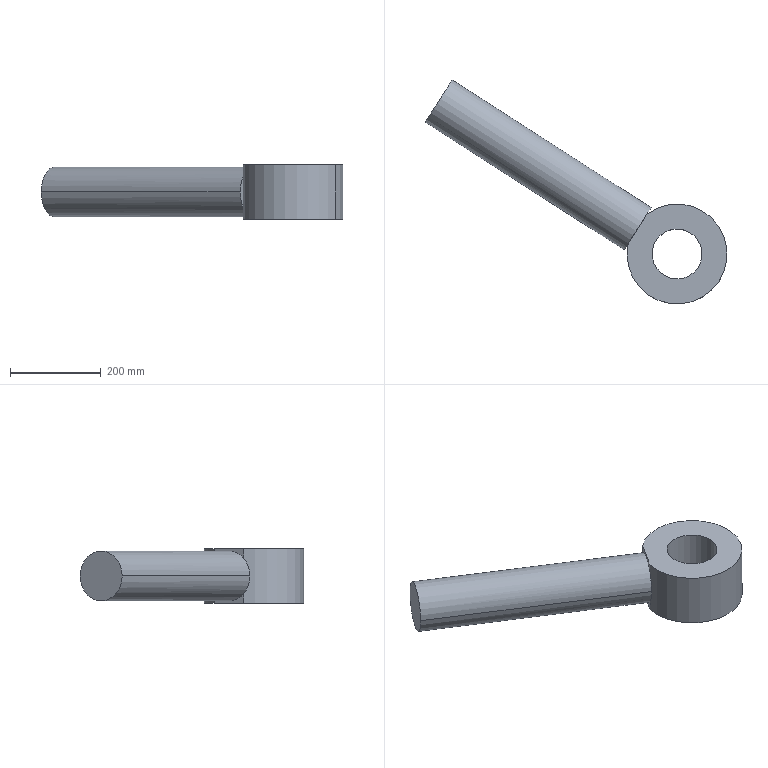Part | SolidWorks | features SplitBody 1 | 1 solid | 13 faces | box 664.027 x 492.763 x 120 mm | volume 8319390 mm3 | plane 7 | cylinder 6 | commonest cylinder face diameters 110 x4 220 x2
STEP:
#1=CARTESIAN_POINT('',(3636.913,574.156,927.5));
#2=VERTEX_POINT('',#1);
#3=CARTESIAN_POINT('',(3696.323,666.733,927.5));
#4=VERTEX_POINT('',#3);
#5=CARTESIAN_POINT('',(3666.618,620.445,927.5));
#6=DIRECTION('',(0.8416,-0.5401,0.));
#7=DIRECTION('',(-0.5401,-0.8416,0.));
#8=AXIS2_PLACEMENT_3D('',#5,#6,#7);
#9=CIRCLE('',#8,55.);
#10=EDGE_CURVE('',#2,#4,#9,.T.);
#11=ORIENTED_EDGE('',*,*,#10,.T.);
#12=CARTESIAN_POINT('',(4133.959,385.887,927.5));
#13=VERTEX_POINT('',#12);
#14=CARTESIAN_POINT('',(3696.323,666.733,927.5));
#15=DIRECTION('',(0.8416,-0.5401,0.));
#16=VECTOR('',#15,1000.);
#17=LINE('',#14,#16);
#18=EDGE_CURVE('',#4,#13,#17,.T.);
#19=ORIENTED_EDGE('',*,*,#18,.T.);
#20=CARTESIAN_POINT('',(4125.109,372.096,888.334));
#21=VERTEX_POINT('',#20);
#22=CARTESIAN_POINT('',(4104.254,339.599,927.5));
#23=DIRECTION('',(-0.8416,0.5401,0.));
#24=DIRECTION('',(-0.5401,-0.8416,0.));
#25=AXIS2_PLACEMENT_3D('',#22,#23,#24);
#26=CIRCLE('',#25,55.);
#27=EDGE_CURVE('',#13,#21,#26,.T.);
#28=ORIENTED_EDGE('',*,*,#27,.T.);
#29=CARTESIAN_POINT('',(4083.4,307.102,888.334));
#30=VERTEX_POINT('',#29);
#31=CARTESIAN_POINT('',(4104.254,339.599,927.5));
#32=DIRECTION('',(-0.8416,0.5401,0.));
#33=DIRECTION('',(-0.5401,-0.8416,0.));
#34=AXIS2_PLACEMENT_3D('',#31,#32,#33);
#35=CIRCLE('',#34,55.);
#36=EDGE_CURVE('',#21,#30,#35,.T.);
#37=ORIENTED_EDGE('',*,*,#36,.T.);
#38=CARTESIAN_POINT('',(4074.55,293.31,927.5));
#39=VERTEX_POINT('',#38);
#40=CARTESIAN_POINT('',(4104.254,339.599,927.5));
#41=DIRECTION('',(-0.8416,0.5401,0.));
#42=DIRECTION('',(-0.5401,-0.8416,0.));
#43=AXIS2_PLACEMENT_3D('',#40,#41,#42);
#44=CIRCLE('',#43,55.);
#45=EDGE_CURVE('',#30,#39,#44,.T.);
#46=ORIENTED_EDGE('',*,*,#45,.T.);
#47=CARTESIAN_POINT('',(3636.913,574.156,927.5));
#48=DIRECTION('',(0.8416,-0.5401,0.));
#49=VECTOR('',#48,1000.);
#50=LINE('',#47,#49);
#51=EDGE_CURVE('',#2,#39,#50,.T.);
#52=ORIENTED_EDGE('',*,*,#51,.F.);
#53=EDGE_LOOP('',(#11,#19,#28,#37,#46,#52));
#54=FACE_OUTER_BOUND('',#53,.T.);
#55=CARTESIAN_POINT('',(3666.618,620.445,927.5));
#56=DIRECTION('',(0.8416,-0.5401,0.));
#57=DIRECTION('',(-0.5401,-0.8416,0.));
#58=AXIS2_PLACEMENT_3D('',#55,#56,#57);
#59=CYLINDRICAL_SURFACE('',#58,55.);
#60=ADVANCED_FACE('',(#54),#59,.T.);
#61=CARTESIAN_POINT('',(4083.4,307.102,867.5));
#62=VERTEX_POINT('',#61);
#63=CARTESIAN_POINT('',(4283.517,224.56,867.5));
#64=VERTEX_POINT('',#63);
#65=CARTESIAN_POINT('',(4190.94,283.97,867.5));
#66=DIRECTION('',(0.,0.,1.));
#67=DIRECTION('',(0.8416,-0.5401,0.));
#68=AXIS2_PLACEMENT_3D('',#65,#66,#67);
#69=CIRCLE('',#68,110.);
#70=EDGE_CURVE('',#62,#64,#69,.T.);
#71=ORIENTED_EDGE('',*,*,#70,.T.);
#72=CARTESIAN_POINT('',(4283.517,224.56,987.5));
#73=VERTEX_POINT('',#72);
#74=CARTESIAN_POINT('',(4283.517,224.56,867.5));
#75=DIRECTION('',(0.,0.,1.));
#76=VECTOR('',#75,1000.);
#77=LINE('',#74,#76);
#78=EDGE_CURVE('',#64,#73,#77,.T.);
#79=ORIENTED_EDGE('',*,*,#78,.T.);
#80=CARTESIAN_POINT('',(4083.4,307.102,987.5));
#81=VERTEX_POINT('',#80);
#82=CARTESIAN_POINT('',(4190.94,283.97,987.5));
#83=DIRECTION('',(0.,0.,-1.));
#84=DIRECTION('',(0.8416,-0.5401,0.));
#85=AXIS2_PLACEMENT_3D('',#82,#83,#84);
#86=CIRCLE('',#85,110.);
#87=EDGE_CURVE('',#73,#81,#86,.T.);
#88=ORIENTED_EDGE('',*,*,#87,.T.);
#89=CARTESIAN_POINT('',(4083.4,307.102,966.666));
#90=VERTEX_POINT('',#89);
#91=CARTESIAN_POINT('',(4083.4,307.102,867.5));
#92=DIRECTION('',(0.,0.,-1.));
#93=VECTOR('',#92,1000.);
#94=LINE('',#91,#93);
#95=EDGE_CURVE('',#81,#90,#94,.T.);
#96=ORIENTED_EDGE('',*,*,#95,.T.);
#97=CARTESIAN_POINT('',(4083.4,307.102,927.5));
#98=DIRECTION('',(0.,0.,-1.));
#99=VECTOR('',#98,1000.);
#100=LINE('',#97,#99);
#101=EDGE_CURVE('',#90,#30,#100,.T.);
#102=ORIENTED_EDGE('',*,*,#101,.T.);
#103=CARTESIAN_POINT('',(4083.4,307.102,867.5));
#104=DIRECTION('',(0.,0.,-1.));
#105=VECTOR('',#104,1000.);
#106=LINE('',#103,#105);
#107=EDGE_CURVE('',#30,#62,#106,.T.);
#108=ORIENTED_EDGE('',*,*,#107,.T.);
#109=EDGE_LOOP('',(#71,#79,#88,#96,#102,#108));
#110=FACE_OUTER_BOUND('',#109,.T.);
#111=CARTESIAN_POINT('',(4190.94,283.97,867.5));
#112=DIRECTION('',(0.,0.,1.));
#113=DIRECTION('',(0.8416,-0.5401,0.));
#114=AXIS2_PLACEMENT_3D('',#111,#112,#113);
#115=CYLINDRICAL_SURFACE('',#114,110.);
#116=ADVANCED_FACE('',(#110),#115,.T.);
#117=CARTESIAN_POINT('',(4144.652,313.675,867.5));
#118=VERTEX_POINT('',#117);
#119=CARTESIAN_POINT('',(4237.229,254.265,867.5));
#120=VERTEX_POINT('',#119);
#121=CARTESIAN_POINT('',(4190.94,283.97,867.5));
#122=DIRECTION('',(0.,0.,1.));
#123=DIRECTION('',(0.8416,-0.5401,0.));
#124=AXIS2_PLACEMENT_3D('',#121,#122,#123);
#125=CIRCLE('',#124,55.);
#126=EDGE_CURVE('',#118,#120,#125,.T.);
#127=ORIENTED_EDGE('',*,*,#126,.F.);
#128=CARTESIAN_POINT('',(4144.652,313.675,987.5));
#129=VERTEX_POINT('',#128);
#130=CARTESIAN_POINT('',(4144.652,313.675,867.5));
#131=DIRECTION('',(0.,0.,1.));
#132=VECTOR('',#131,1000.);
#133=LINE('',#130,#132);
#134=EDGE_CURVE('',#118,#129,#133,.T.);
#135=ORIENTED_EDGE('',*,*,#134,.T.);
#136=CARTESIAN_POINT('',(4237.229,254.265,987.5));
#137=VERTEX_POINT('',#136);
#138=CARTESIAN_POINT('',(4190.94,283.97,987.5));
#139=DIRECTION('',(0.,0.,1.));
#140=DIRECTION('',(0.8416,-0.5401,0.));
#141=AXIS2_PLACEMENT_3D('',#138,#139,#140);
#142=CIRCLE('',#141,55.);
#143=EDGE_CURVE('',#129,#137,#142,.T.);
#144=ORIENTED_EDGE('',*,*,#143,.T.);
#145=CARTESIAN_POINT('',(4237.229,254.265,867.5));
#146=DIRECTION('',(0.,0.,1.));
#147=VECTOR('',#146,1000.);
#148=LINE('',#145,#147);
#149=EDGE_CURVE('',#120,#137,#148,.T.);
#150=ORIENTED_EDGE('',*,*,#149,.F.);
#151=EDGE_LOOP('',(#127,#135,#144,#150));
#152=FACE_OUTER_BOUND('',#151,.T.);
#153=CARTESIAN_POINT('',(4190.94,283.97,867.5));
#154=DIRECTION('',(0.,0.,1.));
#155=DIRECTION('',(0.8416,-0.5401,0.));
#156=AXIS2_PLACEMENT_3D('',#153,#154,#155);
#157=CYLINDRICAL_SURFACE('',#156,55.);
#158=ADVANCED_FACE('',(#152),#157,.F.);
#159=ORIENTED_EDGE('',*,*,#18,.F.);
#160=CARTESIAN_POINT('',(3666.618,620.445,927.5));
#161=DIRECTION('',(0.8416,-0.5401,0.));
#162=DIRECTION('',(-0.5401,-0.8416,0.));
#163=AXIS2_PLACEMENT_3D('',#160,#161,#162);
#164=CIRCLE('',#163,55.);
#165=EDGE_CURVE('',#4,#2,#164,.T.);
#166=ORIENTED_EDGE('',*,*,#165,.T.);
#167=ORIENTED_EDGE('',*,*,#51,.T.);
#168=CARTESIAN_POINT('',(4104.254,339.599,927.5));
#169=DIRECTION('',(-0.8416,0.5401,0.));
#170=DIRECTION('',(-0.5401,-0.8416,0.));
#171=AXIS2_PLACEMENT_3D('',#168,#169,#170);
#172=CIRCLE('',#171,55.);
#173=EDGE_CURVE('',#39,#90,#172,.T.);
#174=ORIENTED_EDGE('',*,*,#173,.T.);
#175=CARTESIAN_POINT('',(4125.109,372.096,966.666));
#176=VERTEX_POINT('',#175);
#177=CARTESIAN_POINT('',(4104.254,339.599,927.5));
#178=DIRECTION('',(-0.8416,0.5401,0.));
#179=DIRECTION('',(-0.5401,-0.8416,0.));
#180=AXIS2_PLACEMENT_3D('',#177,#178,#179);
#181=CIRCLE('',#180,55.);
#182=EDGE_CURVE('',#90,#176,#181,.T.);
#183=ORIENTED_EDGE('',*,*,#182,.T.);
#184=CARTESIAN_POINT('',(4104.254,339.599,927.5));
#185=DIRECTION('',(-0.8416,0.5401,0.));
#186=DIRECTION('',(-0.5401,-0.8416,0.));
#187=AXIS2_PLACEMENT_3D('',#184,#185,#186);
#188=CIRCLE('',#187,55.);
#189=EDGE_CURVE('',#176,#13,#188,.T.);
#190=ORIENTED_EDGE('',*,*,#189,.T.);
#191=EDGE_LOOP('',(#159,#166,#167,#174,#183,#190));
#192=FACE_OUTER_BOUND('',#191,.T.);
#193=CARTESIAN_POINT('',(3666.618,620.445,927.5));
#194=DIRECTION('',(0.8416,-0.5401,0.));
#195=DIRECTION('',(-0.5401,-0.8416,0.));
#196=AXIS2_PLACEMENT_3D('',#193,#194,#195);
#197=CYLINDRICAL_SURFACE('',#196,55.);
#198=ADVANCED_FACE('',(#192),#197,.T.);
#199=ORIENTED_EDGE('',*,*,#101,.F.);
#200=ORIENTED_EDGE('',*,*,#173,.F.);
#201=ORIENTED_EDGE('',*,*,#45,.F.);
#202=EDGE_LOOP('',(#199,#200,#201));
#203=FACE_OUTER_BOUND('',#202,.T.);
#204=CARTESIAN_POINT('',(4104.254,339.599,927.5));
#205=DIRECTION('',(-0.8416,0.5401,0.));
#206=DIRECTION('',(0.5401,0.8416,0.));
#207=AXIS2_PLACEMENT_3D('',#204,#205,#206);
#208=PLANE('',#207);
#209=ADVANCED_FACE('',(#203),#208,.F.);
#210=ORIENTED_EDGE('',*,*,#36,.F.);
#211=CARTESIAN_POINT('',(4125.109,372.096,867.5));
#212=VERTEX_POINT('',#211);
#213=CARTESIAN_POINT('',(4125.109,372.096,867.5));
#214=DIRECTION('',(0.,0.,1.));
#215=VECTOR('',#214,1000.);
#216=LINE('',#213,#215);
#217=EDGE_CURVE('',#212,#21,#216,.T.);
#218=ORIENTED_EDGE('',*,*,#217,.F.);
#219=CARTESIAN_POINT('',(4083.4,307.102,867.5));
#220=DIRECTION('',(0.5401,0.8416,0.));
#221=VECTOR('',#220,1000.);
#222=LINE('',#219,#221);
#223=EDGE_CURVE('',#62,#212,#222,.T.);
#224=ORIENTED_EDGE('',*,*,#223,.F.);
#225=ORIENTED_EDGE('',*,*,#107,.F.);
#226=EDGE_LOOP('',(#210,#218,#224,#225));
#227=FACE_OUTER_BOUND('',#226,.T.);
#228=CARTESIAN_POINT('',(4083.4,307.102,867.5));
#229=DIRECTION('',(0.8416,-0.5401,0.));
#230=DIRECTION('',(-0.5401,-0.8416,0.));
#231=AXIS2_PLACEMENT_3D('',#228,#229,#230);
#232=PLANE('',#231);
#233=ADVANCED_FACE('',(#227),#232,.F.);
#234=ORIENTED_EDGE('',*,*,#189,.F.);
#235=CARTESIAN_POINT('',(4125.109,372.096,927.5));
#236=DIRECTION('',(0.,0.,1.));
#237=VECTOR('',#236,1000.);
#238=LINE('',#235,#237);
#239=EDGE_CURVE('',#21,#176,#238,.T.);
#240=ORIENTED_EDGE('',*,*,#239,.F.);
#241=ORIENTED_EDGE('',*,*,#27,.F.);
#242=EDGE_LOOP('',(#234,#240,#241));
#243=FACE_OUTER_BOUND('',#242,.T.);
#244=CARTESIAN_POINT('',(4104.254,339.599,927.5));
#245=DIRECTION('',(-0.8416,0.5401,0.));
#246=DIRECTION('',(0.5401,0.8416,0.));
#247=AXIS2_PLACEMENT_3D('',#244,#245,#246);
#248=PLANE('',#247);
#249=ADVANCED_FACE('',(#243),#248,.F.);
#250=ORIENTED_EDGE('',*,*,#10,.F.);
#251=ORIENTED_EDGE('',*,*,#165,.F.);
#252=EDGE_LOOP('',(#250,#251));
#253=FACE_OUTER_BOUND('',#252,.T.);
#254=CARTESIAN_POINT('',(3666.618,620.445,927.5));
#255=DIRECTION('',(-0.8416,0.5401,0.));
#256=DIRECTION('',(0.5401,0.8416,0.));
#257=AXIS2_PLACEMENT_3D('',#254,#255,#256);
#258=PLANE('',#257);
#259=ADVANCED_FACE('',(#253),#258,.T.);
#260=ORIENTED_EDGE('',*,*,#182,.F.);
#261=ORIENTED_EDGE('',*,*,#95,.F.);
#262=CARTESIAN_POINT('',(4125.109,372.096,987.5));
#263=VERTEX_POINT('',#262);
#264=CARTESIAN_POINT('',(4083.4,307.102,987.5));
#265=DIRECTION('',(-0.5401,-0.8416,0.));
#266=VECTOR('',#265,1000.);
#267=LINE('',#264,#266);
#268=EDGE_CURVE('',#263,#81,#267,.T.);
#269=ORIENTED_EDGE('',*,*,#268,.F.);
#270=CARTESIAN_POINT('',(4125.109,372.096,867.5));
#271=DIRECTION('',(0.,0.,1.));
#272=VECTOR('',#271,1000.);
#273=LINE('',#270,#272);
#274=EDGE_CURVE('',#176,#263,#273,.T.);
#275=ORIENTED_EDGE('',*,*,#274,.F.);
#276=EDGE_LOOP('',(#260,#261,#269,#275));
#277=FACE_OUTER_BOUND('',#276,.T.);
#278=CARTESIAN_POINT('',(4083.4,307.102,867.5));
#279=DIRECTION('',(0.8416,-0.5401,0.));
#280=DIRECTION('',(-0.5401,-0.8416,0.));
#281=AXIS2_PLACEMENT_3D('',#278,#279,#280);
#282=PLANE('',#281);
#283=ADVANCED_FACE('',(#277),#282,.F.);
#284=ORIENTED_EDGE('',*,*,#78,.F.);
#285=CARTESIAN_POINT('',(4190.94,283.97,867.5));
#286=DIRECTION('',(0.,0.,1.));
#287=DIRECTION('',(0.8416,-0.5401,0.));
#288=AXIS2_PLACEMENT_3D('',#285,#286,#287);
#289=CIRCLE('',#288,110.);
#290=EDGE_CURVE('',#64,#212,#289,.T.);
#291=ORIENTED_EDGE('',*,*,#290,.T.);
#292=ORIENTED_EDGE('',*,*,#217,.T.);
#293=ORIENTED_EDGE('',*,*,#239,.T.);
#294=ORIENTED_EDGE('',*,*,#274,.T.);
#295=CARTESIAN_POINT('',(4190.94,283.97,987.5));
#296=DIRECTION('',(0.,0.,-1.));
#297=DIRECTION('',(0.8416,-0.5401,0.));
#298=AXIS2_PLACEMENT_3D('',#295,#296,#297);
#299=CIRCLE('',#298,110.);
#300=EDGE_CURVE('',#263,#73,#299,.T.);
#301=ORIENTED_EDGE('',*,*,#300,.T.);
#302=EDGE_LOOP('',(#284,#291,#292,#293,#294,#301));
#303=FACE_OUTER_BOUND('',#302,.T.);
#304=CARTESIAN_POINT('',(4190.94,283.97,867.5));
#305=DIRECTION('',(0.,0.,1.));
#306=DIRECTION('',(0.8416,-0.5401,0.));
#307=AXIS2_PLACEMENT_3D('',#304,#305,#306);
#308=CYLINDRICAL_SURFACE('',#307,110.);
#309=ADVANCED_FACE('',(#303),#308,.T.);
#310=CARTESIAN_POINT('',(4190.94,283.97,867.5));
#311=DIRECTION('',(0.,0.,1.));
#312=DIRECTION('',(0.8416,-0.5401,0.));
#313=AXIS2_PLACEMENT_3D('',#310,#311,#312);
#314=CIRCLE('',#313,55.);
#315=EDGE_CURVE('',#120,#118,#314,.T.);
#316=ORIENTED_EDGE('',*,*,#315,.T.);
#317=ORIENTED_EDGE('',*,*,#126,.T.);
#318=EDGE_LOOP('',(#316,#317));
#319=FACE_BOUND('',#318,.T.);
#320=ORIENTED_EDGE('',*,*,#70,.F.);
#321=ORIENTED_EDGE('',*,*,#223,.T.);
#322=ORIENTED_EDGE('',*,*,#290,.F.);
#323=EDGE_LOOP('',(#320,#321,#322));
#324=FACE_OUTER_BOUND('',#323,.T.);
#325=CARTESIAN_POINT('',(4190.94,283.97,867.5));
#326=DIRECTION('',(0.,0.,-1.));
#327=DIRECTION('',(-0.8416,0.5401,0.));
#328=AXIS2_PLACEMENT_3D('',#325,#326,#327);
#329=PLANE('',#328);
#330=ADVANCED_FACE('',(#319,#324),#329,.T.);
#331=CARTESIAN_POINT('',(4190.94,283.97,987.5));
#332=DIRECTION('',(0.,0.,1.));
#333=DIRECTION('',(0.8416,-0.5401,0.));
#334=AXIS2_PLACEMENT_3D('',#331,#332,#333);
#335=CIRCLE('',#334,55.);
#336=EDGE_CURVE('',#137,#129,#335,.T.);
#337=ORIENTED_EDGE('',*,*,#336,.F.);
#338=ORIENTED_EDGE('',*,*,#143,.F.);
#339=EDGE_LOOP('',(#337,#338));
#340=FACE_BOUND('',#339,.T.);
#341=ORIENTED_EDGE('',*,*,#268,.T.);
#342=ORIENTED_EDGE('',*,*,#87,.F.);
#343=ORIENTED_EDGE('',*,*,#300,.F.);
#344=EDGE_LOOP('',(#341,#342,#343));
#345=FACE_OUTER_BOUND('',#344,.T.);
#346=CARTESIAN_POINT('',(4190.94,283.97,987.5));
#347=DIRECTION('',(0.,0.,-1.));
#348=DIRECTION('',(-0.8416,0.5401,0.));
#349=AXIS2_PLACEMENT_3D('',#346,#347,#348);
#350=PLANE('',#349);
#351=ADVANCED_FACE('',(#340,#345),#350,.F.);
#352=ORIENTED_EDGE('',*,*,#134,.F.);
#353=ORIENTED_EDGE('',*,*,#315,.F.);
#354=ORIENTED_EDGE('',*,*,#149,.T.);
#355=ORIENTED_EDGE('',*,*,#336,.T.);
#356=EDGE_LOOP('',(#352,#353,#354,#355));
#357=FACE_OUTER_BOUND('',#356,.T.);
#358=CARTESIAN_POINT('',(4190.94,283.97,867.5));
#359=DIRECTION('',(0.,0.,1.));
#360=DIRECTION('',(0.8416,-0.5401,0.));
#361=AXIS2_PLACEMENT_3D('',#358,#359,#360);
#362=CYLINDRICAL_SURFACE('',#361,55.);
#363=ADVANCED_FACE('',(#357),#362,.F.);
#364=CLOSED_SHELL('',(#60,#116,#158,#198,#209,#233,#249,#259,#283,#309,#330,#351,#363));
#365=MANIFOLD_SOLID_BREP('',#364);
#366=CARTESIAN_POINT('',(0.,0.,0.));
#367=DIRECTION('',(0.,0.,1.));
#368=DIRECTION('',(1.,0.,0.));
#369=AXIS2_PLACEMENT_3D('',#366,#367,#368);
#370=(LENGTH_UNIT()NAMED_UNIT(*)SI_UNIT(.MILLI.,.METRE.));
#371=UNCERTAINTY_MEASURE_WITH_UNIT(LENGTH_MEASURE(0.00001),#370,'','');
#372=(NAMED_UNIT(*)PLANE_ANGLE_UNIT()SI_UNIT($,.RADIAN.));
#373=(NAMED_UNIT(*)SI_UNIT($,.STERADIAN.)SOLID_ANGLE_UNIT());
#374=(GEOMETRIC_REPRESENTATION_CONTEXT(3)GLOBAL_UNCERTAINTY_ASSIGNED_CONTEXT((#371))GLOBAL_UNIT_ASSIGNED_CONTEXT((#370,#372,#373))REPRESENTATION_CONTEXT('',''));
#375=ADVANCED_BREP_SHAPE_REPRESENTATION('',(#365,#369),#374);